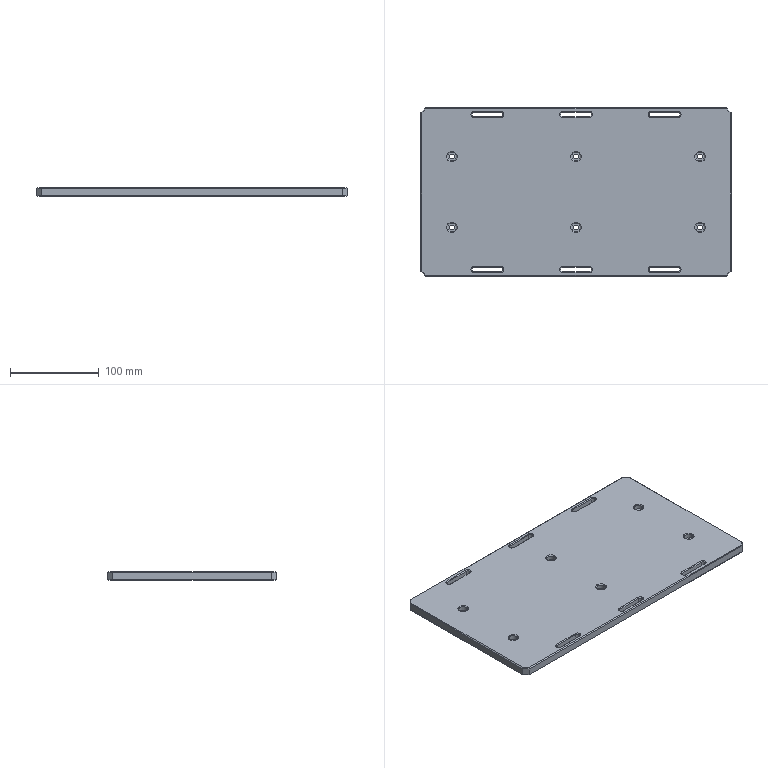Part | STEP file | 1 solid | 170 faces | box 350 x 190 x 10 mm | volume 648871 mm3 | plane 68 | cone 60 | cylinder 42 | commonest cylinder face diameters 5.2 x18 5.5 x12 10 x12